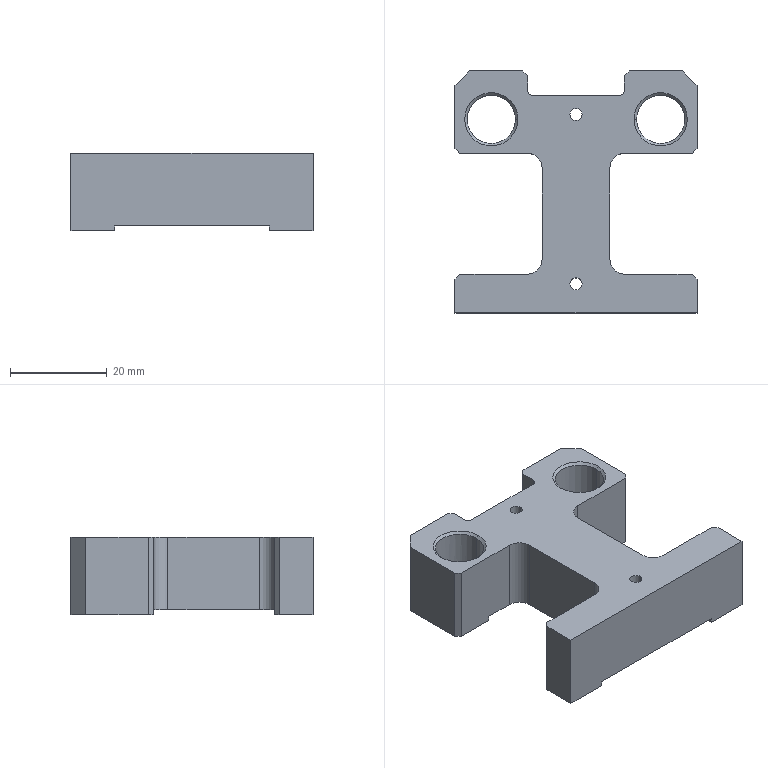Part | SolidWorks | features Chamfer 3, ICE 3, Fillet 2, HoleWzd 2, Extrusion 1 | 1 solid | 61 faces | box 50 x 50 x 16 mm | volume 20170 mm3 | plane 36 | cylinder 18 | cone 7 | commonest cylinder face diameters 2.5 x4 3.3 x4 6 x4 10 x4 2 x2